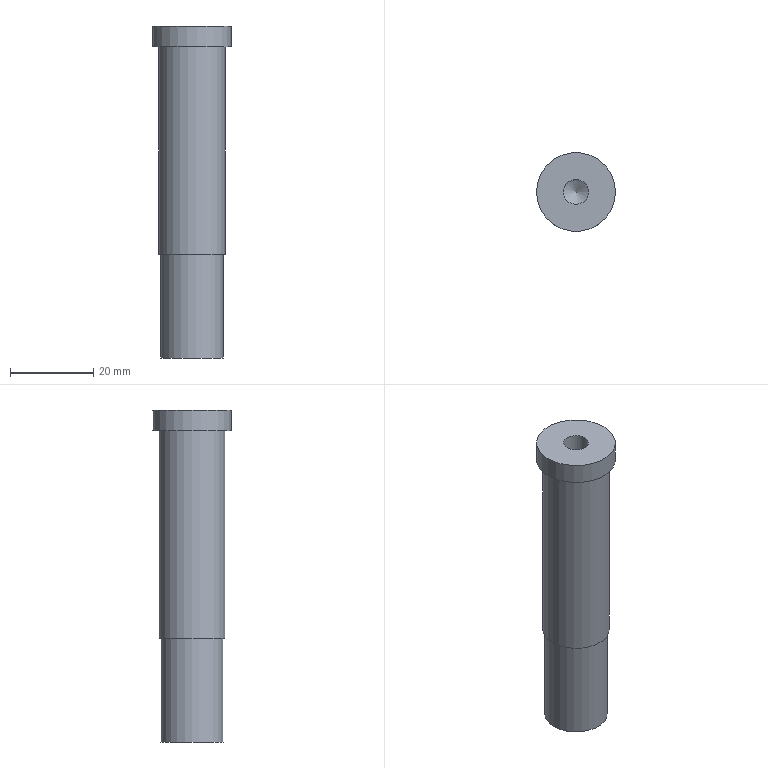Part | NX | features solid 2 | 1 solid | 9 faces | box 19 x 19 x 80 mm | volume 15534 mm3 | cylinder 4 | plane 4 | cone 1 | commonest cylinder face diameters 6 x1 15.05 x1 16 x1 19 x1
STEP:
#1=CARTESIAN_POINT('',(-676.997,-184.057,50.));
#2=VERTEX_POINT('',#1);
#3=CARTESIAN_POINT('',(-684.997,-184.057,50.));
#4=DIRECTION('',(0.,0.,1.));
#5=DIRECTION('',(1.,0.,0.));
#6=AXIS2_PLACEMENT_3D('',#3,#4,#5);
#7=CIRCLE('',#6,8.);
#8=EDGE_CURVE('',#2,#2,#7,.T.);
#9=ORIENTED_EDGE('',*,*,#8,.T.);
#10=EDGE_LOOP('',(#9));
#11=FACE_BOUND('',#10,.T.);
#12=CARTESIAN_POINT('',(-676.997,-184.057,100.));
#13=VERTEX_POINT('',#12);
#14=CARTESIAN_POINT('',(-684.997,-184.057,100.));
#15=DIRECTION('',(0.,0.,1.));
#16=DIRECTION('',(1.,0.,0.));
#17=AXIS2_PLACEMENT_3D('',#14,#15,#16);
#18=CIRCLE('',#17,8.);
#19=EDGE_CURVE('',#13,#13,#18,.T.);
#20=ORIENTED_EDGE('',*,*,#19,.F.);
#21=EDGE_LOOP('',(#20));
#22=FACE_BOUND('',#21,.T.);
#23=CARTESIAN_POINT('',(-684.997,-184.057,105.));
#24=DIRECTION('',(0.,0.,-1.));
#25=DIRECTION('',(-1.,0.,0.));
#26=AXIS2_PLACEMENT_3D('',#23,#24,#25);
#27=CYLINDRICAL_SURFACE('',#26,8.);
#28=ADVANCED_FACE('',(#11,#22),#27,.T.);
#29=CARTESIAN_POINT('',(-677.472,-184.057,50.));
#30=VERTEX_POINT('',#29);
#31=CARTESIAN_POINT('',(-684.997,-184.057,50.));
#32=DIRECTION('',(0.,0.,1.));
#33=DIRECTION('',(1.,0.,0.));
#34=AXIS2_PLACEMENT_3D('',#31,#32,#33);
#35=CIRCLE('',#34,7.525);
#36=EDGE_CURVE('',#30,#30,#35,.T.);
#37=ORIENTED_EDGE('',*,*,#36,.T.);
#38=EDGE_LOOP('',(#37));
#39=FACE_BOUND('',#38,.T.);
#40=ORIENTED_EDGE('',*,*,#8,.F.);
#41=EDGE_LOOP('',(#40));
#42=FACE_BOUND('',#41,.T.);
#43=CARTESIAN_POINT('',(-684.997,-184.057,50.));
#44=DIRECTION('',(0.,0.,1.));
#45=DIRECTION('',(1.,0.,0.));
#46=AXIS2_PLACEMENT_3D('',#43,#44,#45);
#47=PLANE('',#46);
#48=ADVANCED_FACE('',(#39,#42),#47,.F.);
#49=CARTESIAN_POINT('',(-675.497,-184.057,100.));
#50=VERTEX_POINT('',#49);
#51=CARTESIAN_POINT('',(-684.997,-184.057,100.));
#52=DIRECTION('',(0.,0.,1.));
#53=DIRECTION('',(1.,0.,0.));
#54=AXIS2_PLACEMENT_3D('',#51,#52,#53);
#55=CIRCLE('',#54,9.5);
#56=EDGE_CURVE('',#50,#50,#55,.T.);
#57=ORIENTED_EDGE('',*,*,#56,.F.);
#58=EDGE_LOOP('',(#57));
#59=FACE_BOUND('',#58,.T.);
#60=ORIENTED_EDGE('',*,*,#19,.T.);
#61=EDGE_LOOP('',(#60));
#62=FACE_BOUND('',#61,.T.);
#63=CARTESIAN_POINT('',(-684.997,-184.057,100.));
#64=DIRECTION('',(0.,0.,1.));
#65=DIRECTION('',(1.,0.,0.));
#66=AXIS2_PLACEMENT_3D('',#63,#64,#65);
#67=PLANE('',#66);
#68=ADVANCED_FACE('',(#59,#62),#67,.F.);
#69=ORIENTED_EDGE('',*,*,#56,.T.);
#70=EDGE_LOOP('',(#69));
#71=FACE_BOUND('',#70,.T.);
#72=CARTESIAN_POINT('',(-675.497,-184.057,105.));
#73=VERTEX_POINT('',#72);
#74=CARTESIAN_POINT('',(-684.997,-184.057,105.));
#75=DIRECTION('',(0.,0.,1.));
#76=DIRECTION('',(1.,0.,0.));
#77=AXIS2_PLACEMENT_3D('',#74,#75,#76);
#78=CIRCLE('',#77,9.5);
#79=EDGE_CURVE('',#73,#73,#78,.T.);
#80=ORIENTED_EDGE('',*,*,#79,.F.);
#81=EDGE_LOOP('',(#80));
#82=FACE_BOUND('',#81,.T.);
#83=CARTESIAN_POINT('',(-684.997,-184.057,100.));
#84=DIRECTION('',(0.,0.,1.));
#85=DIRECTION('',(1.,0.,0.));
#86=AXIS2_PLACEMENT_3D('',#83,#84,#85);
#87=CYLINDRICAL_SURFACE('',#86,9.5);
#88=ADVANCED_FACE('',(#71,#82),#87,.T.);
#89=CARTESIAN_POINT('',(-687.997,-184.057,105.));
#90=VERTEX_POINT('',#89);
#91=CARTESIAN_POINT('',(-684.997,-184.057,105.));
#92=DIRECTION('',(0.,0.,-1.));
#93=DIRECTION('',(-1.,0.,0.));
#94=AXIS2_PLACEMENT_3D('',#91,#92,#93);
#95=CIRCLE('',#94,3.);
#96=EDGE_CURVE('',#90,#90,#95,.T.);
#97=ORIENTED_EDGE('',*,*,#96,.T.);
#98=EDGE_LOOP('',(#97));
#99=FACE_BOUND('',#98,.T.);
#100=ORIENTED_EDGE('',*,*,#79,.T.);
#101=EDGE_LOOP('',(#100));
#102=FACE_BOUND('',#101,.T.);
#103=CARTESIAN_POINT('',(-684.997,-184.057,105.));
#104=DIRECTION('',(0.,0.,1.));
#105=DIRECTION('',(1.,0.,0.));
#106=AXIS2_PLACEMENT_3D('',#103,#104,#105);
#107=PLANE('',#106);
#108=ADVANCED_FACE('',(#99,#102),#107,.T.);
#109=CARTESIAN_POINT('',(-677.472,-184.057,25.));
#110=VERTEX_POINT('',#109);
#111=CARTESIAN_POINT('',(-684.997,-184.057,25.));
#112=DIRECTION('',(0.,0.,1.));
#113=DIRECTION('',(1.,0.,0.));
#114=AXIS2_PLACEMENT_3D('',#111,#112,#113);
#115=CIRCLE('',#114,7.525);
#116=EDGE_CURVE('',#110,#110,#115,.T.);
#117=ORIENTED_EDGE('',*,*,#116,.T.);
#118=EDGE_LOOP('',(#117));
#119=FACE_BOUND('',#118,.T.);
#120=ORIENTED_EDGE('',*,*,#36,.F.);
#121=EDGE_LOOP('',(#120));
#122=FACE_BOUND('',#121,.T.);
#123=CARTESIAN_POINT('',(-684.997,-184.057,25.));
#124=DIRECTION('',(0.,0.,1.));
#125=DIRECTION('',(1.,0.,0.));
#126=AXIS2_PLACEMENT_3D('',#123,#124,#125);
#127=CYLINDRICAL_SURFACE('',#126,7.525);
#128=ADVANCED_FACE('',(#119,#122),#127,.T.);
#129=ORIENTED_EDGE('',*,*,#116,.F.);
#130=EDGE_LOOP('',(#129));
#131=FACE_BOUND('',#130,.T.);
#132=CARTESIAN_POINT('',(-684.997,-184.057,25.));
#133=DIRECTION('',(0.,0.,1.));
#134=DIRECTION('',(1.,0.,0.));
#135=AXIS2_PLACEMENT_3D('',#132,#133,#134);
#136=PLANE('',#135);
#137=ADVANCED_FACE('',(#131),#136,.F.);
#138=CARTESIAN_POINT('',(-687.997,-184.057,92.));
#139=VERTEX_POINT('',#138);
#140=CARTESIAN_POINT('',(-684.997,-184.057,92.));
#141=DIRECTION('',(0.,0.,-1.));
#142=DIRECTION('',(-1.,0.,0.));
#143=AXIS2_PLACEMENT_3D('',#140,#141,#142);
#144=CIRCLE('',#143,3.);
#145=EDGE_CURVE('',#139,#139,#144,.T.);
#146=ORIENTED_EDGE('',*,*,#145,.F.);
#147=EDGE_LOOP('',(#146));
#148=FACE_BOUND('',#147,.T.);
#149=CARTESIAN_POINT('',(-684.997,-184.057,90.268));
#150=VERTEX_POINT('',#149);
#151=VERTEX_LOOP('',#150);
#152=FACE_BOUND('',#151,.T.);
#153=CARTESIAN_POINT('',(-684.997,-184.057,92.));
#154=DIRECTION('',(0.,0.,1.));
#155=DIRECTION('',(1.,0.,0.));
#156=AXIS2_PLACEMENT_3D('',#153,#154,#155);
#157=CONICAL_SURFACE('',#156,3.,1.047);
#158=ADVANCED_FACE('',(#148,#152),#157,.F.);
#159=ORIENTED_EDGE('',*,*,#145,.T.);
#160=EDGE_LOOP('',(#159));
#161=FACE_BOUND('',#160,.T.);
#162=ORIENTED_EDGE('',*,*,#96,.F.);
#163=EDGE_LOOP('',(#162));
#164=FACE_BOUND('',#163,.T.);
#165=CARTESIAN_POINT('',(-684.997,-184.057,105.));
#166=DIRECTION('',(0.,0.,-1.));
#167=DIRECTION('',(-1.,0.,0.));
#168=AXIS2_PLACEMENT_3D('',#165,#166,#167);
#169=CYLINDRICAL_SURFACE('',#168,3.);
#170=ADVANCED_FACE('',(#161,#164),#169,.F.);
#171=CLOSED_SHELL('',(#28,#48,#68,#88,#108,#128,#137,#158,#170));
#172=MANIFOLD_SOLID_BREP('',#171);
#173=(LENGTH_UNIT()NAMED_UNIT(*)SI_UNIT(.MILLI.,.METRE.));
#174=UNCERTAINTY_MEASURE_WITH_UNIT(LENGTH_MEASURE(0.00001),#173,'','');
#175=(NAMED_UNIT(*)PLANE_ANGLE_UNIT()SI_UNIT($,.RADIAN.));
#176=(NAMED_UNIT(*)SI_UNIT($,.STERADIAN.)SOLID_ANGLE_UNIT());
#177=(GEOMETRIC_REPRESENTATION_CONTEXT(3)GLOBAL_UNCERTAINTY_ASSIGNED_CONTEXT((#174))GLOBAL_UNIT_ASSIGNED_CONTEXT((#173,#175,#176))REPRESENTATION_CONTEXT('',''));
#178=ADVANCED_BREP_SHAPE_REPRESENTATION('',(#172),#177);